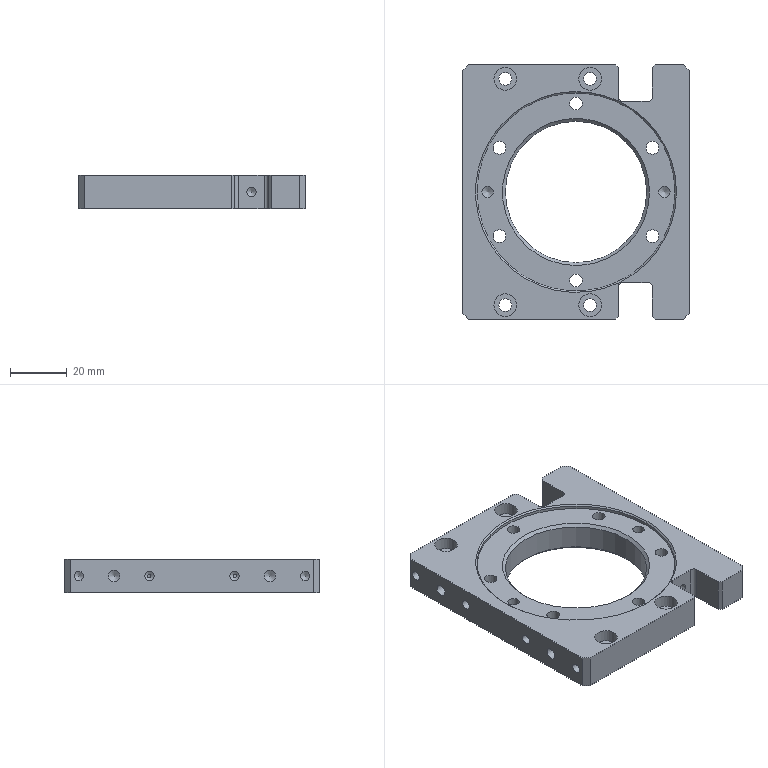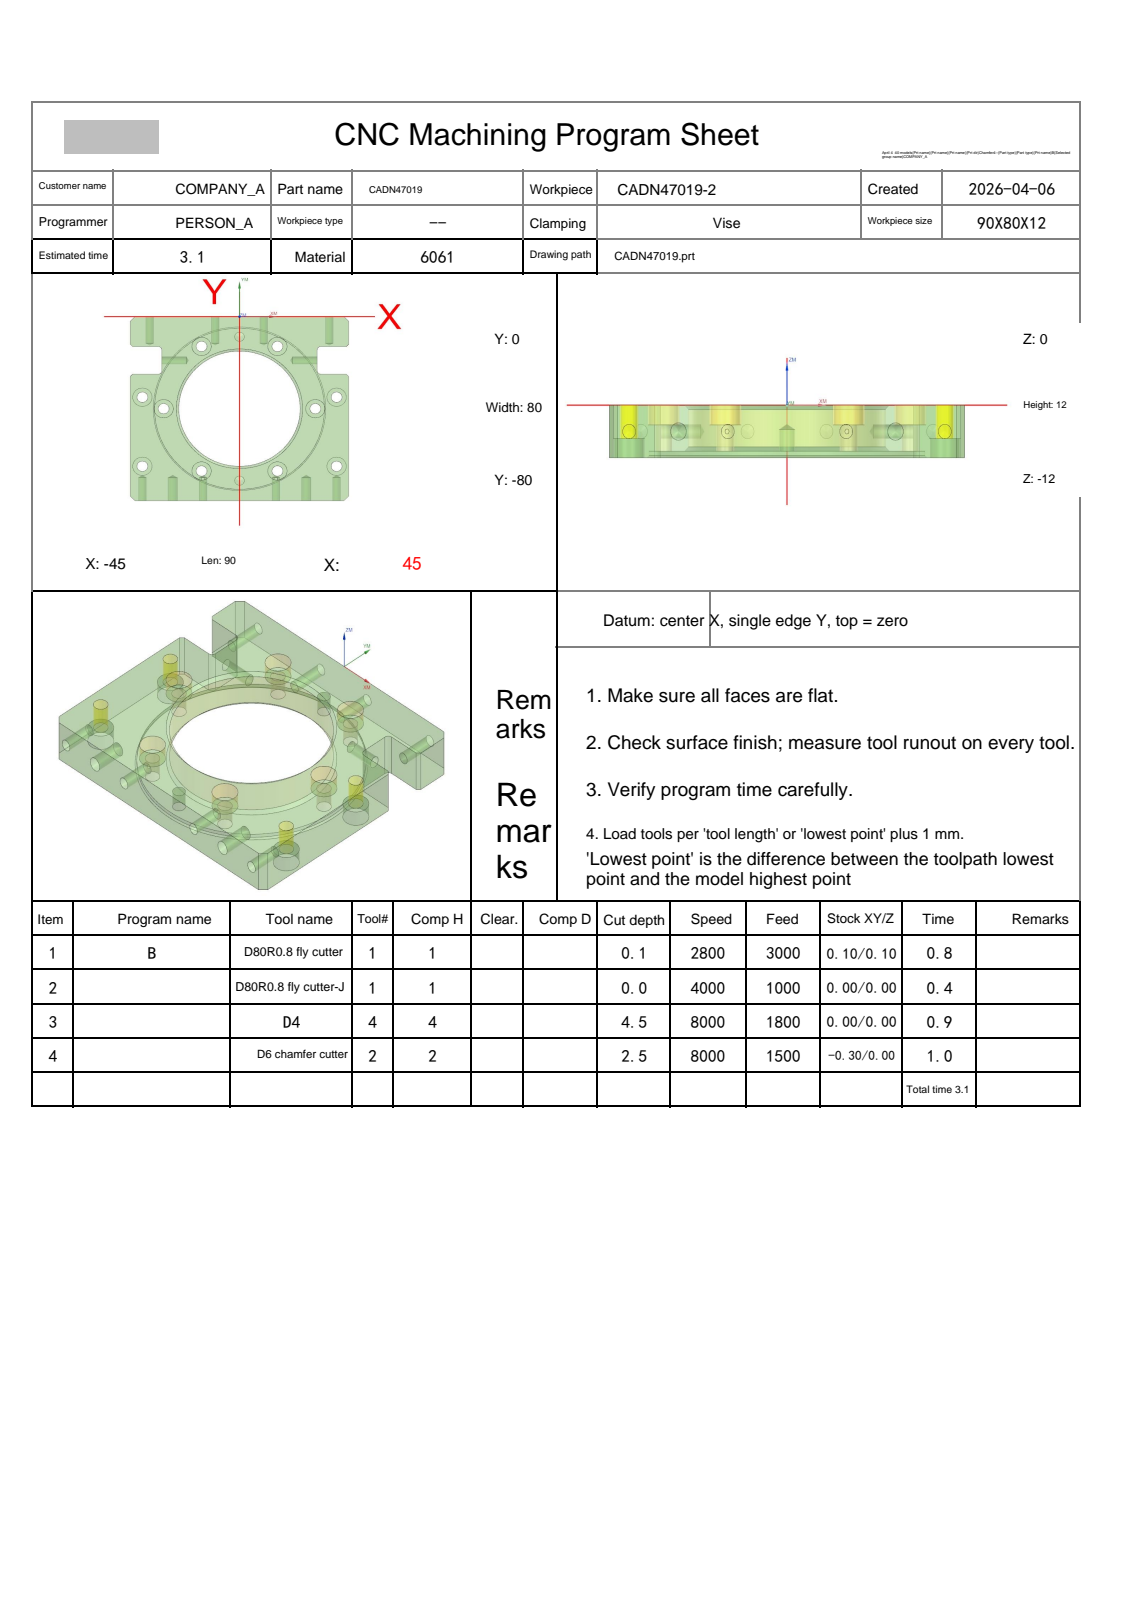NC program | NX | posted by the shop | part box 80 x 90 x 12 mm
Whole program:
%
O0001
(Machine time: 3.82 MIN)
(===Total Tool:3===)
(T1=D80R0.8 fly cutter D=80.  R=0.8  D-  H01 Z=0.    )
(T4=D4      D=4.   R=0.   D-  H04 Z=-4.5  )
(T2=D6 chamfer cutter   D=6.   R=0.   D-  H02 Z=-2.55 )
G80 G90 G17 G49 G40
G91 G28 Z0
M01
N1 T01 M06
(D80R0.8 fly cutter  D=80. R=0.8 H=01 ce=0.10 di=0.10)
G00 G90 G54 X-97.097 Y-23.903 M03 S2800
G43 H01 Z20.
M08
Z4.35
G01 Z2.35 F3000.
X-85.097
X77.897
G02 X85.097 Y-31.103 I0.0 J-7.2
G01 Y-40.737
G02 X77.097 Y-48.737 I-8. J0.0
G01 X-85.097
X-97.097
Z4.35
G00 Y-23.903
Z3.9
G01 Z1.9
X-85.097
X77.897
G02 X85.097 Y-31.103 I0.0 J-7.2
G01 Y-40.737
G02 X77.097 Y-48.737 I-8. J0.0
G01 X-85.097
X-97.097
Z3.9
G00 Y-23.903
Z3.45
G01 Z1.45
X-85.097
X77.897
G02 X85.097 Y-31.103 I0.0 J-7.2
G01 Y-40.737
G02 X77.097 Y-48.737 I-8. J0.0
G01 X-85.097
X-97.097
Z3.45
G00 Y-23.903
Z3.
G01 Z1.
X-85.097
X77.897
G02 X85.097 Y-31.103 I0.0 J-7.2
G01 Y-40.737
G02 X77.097 Y-48.737 I-8. J0.0
G01 X-85.097
X-97.097
Z3.
G00 Y-23.903
Z2.55
G01 Z.55
X-85.097
X77.897
G02 X85.097 Y-31.103 I0.0 J-7.2
G01 Y-40.737
G02 X77.097 Y-48.737 I-8. J0.0
G01 X-85.097
X-97.097
Z2.55
G00 Y-23.903
Z2.1
G01 Z.1
X-85.097
X77.897
G02 X85.097 Y-31.103 I0.0 J-7.2
G01 Y-40.737
G02 X77.097 Y-48.737 I-8. J0.0
G01 X-85.097
X-97.097
Z2.1
G00 Z20.
G91 G28 Z0.0
M05
M09
G91 G28 Z0.0
M01
N2 T01 M06
(D80R0.8 fly cutter-J  D=80. R=0.8 H=01 ce=0.00 di=0.00)
G00 G90 G54 X-96.999 Y-24.001 M03 S4000
G43 H01 Z20.
M08
Z2.
G01 Z0.0 F1000.
X-84.999
X77.002
G02 X84.999 Y-31.998 I-.003 J-8.
G01 Y-41.439
G02 X77.799 Y-48.639 I-7.2 J0.0
G01 X-84.999
X-96.999
Z2.
G00 Z20.
G91 G28 Z0.0
M05
M09
G91 G28 Z0.0
M01
N3 T04 M06
(D4  D=4. R=0. H=04 ce=0.07 di=0.00)
G00 G90 G54 X15.625 Y-12.937 M03 S8000
G43 H04 Z20.
M08
Z.3
G03 X16.59 Y-11.972 I0.0 J.965 F1800.
X15.625 Y-11.007 I-.965 J0.0
X15.625 Y-11.007 Z-.05 I0.0 J-1.93
X15.625 Y-11.007 Z-.4 I0.0 J-1.93
X15.625 Y-11.007 Z-.75 I0.0 J-1.93
X15.625 Y-11.007 Z-1.1 I0.0 J-1.93
X15.625 Y-11.007 Z-1.45 I0.0 J-1.93
X15.625 Y-11.007 Z-1.8 I0.0 J-1.93
X15.625 Y-11.007 Z-2.15 I0.0 J-1.93
X15.625 Y-11.007 Z-2.5 I0.0 J-1.93
X15.625 Y-11.007 Z-2.85 I0.0 J-1.93
X15.625 Y-11.007 Z-3.2 I0.0 J-1.93
X15.625 Y-11.007 Z-3.55 I0.0 J-1.93
X15.625 Y-11.007 Z-3.9 I0.0 J-1.93
X15.625 Y-11.007 Z-4.25 I0.0 J-1.93
X17.507 Y-13.366 Z-4.5 I0.0 J-1.93
X17.555 Y-12.937 I-1.882 J.429
X15.625 Y-11.007 I-1.93 J0.0
X13.695 Y-12.937 I0.0 J-1.93
X15.625 Y-14.867 I1.93 J0.0
X17.507 Y-13.366 I0.0 J1.93
X17.531 Y-13.151 I-.941 J.215
X16.566 Y-12.186 I-.965 J0.0
X15.625 Y-12.937 I0.0 J-.965
G00 Z20.
X-15.625
Z.3
G03 X-14.66 Y-11.972 I0.0 J.965
X-15.625 Y-11.007 I-.965 J0.0
X-15.625 Y-11.007 Z-.05 I0.0 J-1.93
X-15.625 Y-11.007 Z-.4 I0.0 J-1.93
X-15.625 Y-11.007 Z-.75 I0.0 J-1.93
X-15.625 Y-11.007 Z-1.1 I0.0 J-1.93
X-15.625 Y-11.007 Z-1.45 I0.0 J-1.93
X-15.625 Y-11.007 Z-1.8 I0.0 J-1.93
X-15.625 Y-11.007 Z-2.15 I0.0 J-1.93
X-15.625 Y-11.007 Z-2.5 I0.0 J-1.93
X-15.625 Y-11.007 Z-2.85 I0.0 J-1.93
X-15.625 Y-11.007 Z-3.2 I0.0 J-1.93
X-15.625 Y-11.007 Z-3.55 I0.0 J-1.93
X-15.625 Y-11.007 Z-3.9 I0.0 J-1.93
X-15.625 Y-11.007 Z-4.25 I0.0 J-1.93
X-13.743 Y-13.366 Z-4.5 I0.0 J-1.93
X-13.695 Y-12.937 I-1.882 J.429
X-15.625 Y-11.007 I-1.93 J0.0
X-17.555 Y-12.937 I0.0 J-1.93
X-15.625 Y-14.867 I1.93 J0.0
X-13.743 Y-13.366 I0.0 J1.93
X-13.719 Y-13.151 I-.941 J.215
X-14.684 Y-12.186 I-.965 J0.0
X-15.625 Y-12.937 I0.0 J-.965
G00 Z20.
X-31.25 Y-40.
Z.3
G03 X-30.285 Y-39.035 I0.0 J.965
X-31.25 Y-38.07 I-.965 J0.0
X-31.25 Y-38.07 Z-.05 I0.0 J-1.93
X-31.25 Y-38.07 Z-.4 I0.0 J-1.93
X-31.25 Y-38.07 Z-.75 I0.0 J-1.93
X-31.25 Y-38.07 Z-1.1 I0.0 J-1.93
X-31.25 Y-38.07 Z-1.45 I0.0 J-1.93
X-31.25 Y-38.07 Z-1.8 I0.0 J-1.93
X-31.25 Y-38.07 Z-2.15 I0.0 J-1.93
X-31.25 Y-38.07 Z-2.5 I0.0 J-1.93
X-31.25 Y-38.07 Z-2.85 I0.0 J-1.93
X-31.25 Y-38.07 Z-3.2 I0.0 J-1.93
X-31.25 Y-38.07 Z-3.55 I0.0 J-1.93
X-31.25 Y-38.07 Z-3.9 I0.0 J-1.93
X-31.25 Y-38.07 Z-4.25 I0.0 J-1.93
X-29.368 Y-40.429 Z-4.5 I0.0 J-1.93
X-29.32 Y-40. I-1.882 J.429
X-31.25 Y-38.07 I-1.93 J0.0
X-33.18 Y-40. I0.0 J-1.93
X-31.25 Y-41.93 I1.93 J0.0
X-29.368 Y-40.429 I0.0 J1.93
X-29.344 Y-40.215 I-.941 J.215
X-30.309 Y-39.25 I-.965 J0.0
X-31.25 Y-40. I0.0 J-.965
G00 Z20.
X-15.625 Y-67.063
Z.3
G03 X-14.66 Y-66.098 I0.0 J.965
X-15.625 Y-65.133 I-.965 J0.0
X-15.625 Y-65.133 Z-.05 I0.0 J-1.93
X-15.625 Y-65.133 Z-.4 I0.0 J-1.93
X-15.625 Y-65.133 Z-.75 I0.0 J-1.93
X-15.625 Y-65.133 Z-1.1 I0.0 J-1.93
X-15.625 Y-65.133 Z-1.45 I0.0 J-1.93
X-15.625 Y-65.133 Z-1.8 I0.0 J-1.93
X-15.625 Y-65.133 Z-2.15 I0.0 J-1.93
X-15.625 Y-65.133 Z-2.5 I0.0 J-1.93
X-15.625 Y-65.133 Z-2.85 I0.0 J-1.93
X-15.625 Y-65.133 Z-3.2 I0.0 J-1.93
X-15.625 Y-65.133 Z-3.55 I0.0 J-1.93
X-15.625 Y-65.133 Z-3.9 I0.0 J-1.93
X-15.625 Y-65.133 Z-4.25 I0.0 J-1.93
X-13.743 Y-67.493 Z-4.5 I0.0 J-1.93
X-13.695 Y-67.063 I-1.882 J.429
X-15.625 Y-65.133 I-1.93 J0.0
X-17.555 Y-67.063 I0.0 J-1.93
X-15.625 Y-68.993 I1.93 J0.0
X-13.743 Y-67.493 I0.0 J1.93
X-13.719 Y-67.278 I-.941 J.215
X-14.684 Y-66.313 I-.965 J0.0
X-15.625 Y-67.063 I0.0 J-.965
G00 Z20.
X15.625
Z.3
G03 X16.59 Y-66.098 I0.0 J.965
X15.625 Y-65.133 I-.965 J0.0
X15.625 Y-65.133 Z-.05 I0.0 J-1.93
X15.625 Y-65.133 Z-.4 I0.0 J-1.93
X15.625 Y-65.133 Z-.75 I0.0 J-1.93
X15.625 Y-65.133 Z-1.1 I0.0 J-1.93
X15.625 Y-65.133 Z-1.45 I0.0 J-1.93
X15.625 Y-65.133 Z-1.8 I0.0 J-1.93
X15.625 Y-65.133 Z-2.15 I0.0 J-1.93
X15.625 Y-65.133 Z-2.5 I0.0 J-1.93
X15.625 Y-65.133 Z-2.85 I0.0 J-1.93
X15.625 Y-65.133 Z-3.2 I0.0 J-1.93
X15.625 Y-65.133 Z-3.55 I0.0 J-1.93
X15.625 Y-65.133 Z-3.9 I0.0 J-1.93
X15.625 Y-65.133 Z-4.25 I0.0 J-1.93
X17.507 Y-67.493 Z-4.5 I0.0 J-1.93
X17.555 Y-67.063 I-1.882 J.429
X15.625 Y-65.133 I-1.93 J0.0
X13.695 Y-67.063 I0.0 J-1.93
X15.625 Y-68.993 I1.93 J0.0
X17.507 Y-67.493 I0.0 J1.93
X17.531 Y-67.278 I-.941 J.215
X16.566 Y-66.313 I-.965 J0.0
X15.625 Y-67.063 I0.0 J-.965
G00 Z20.
X31.25 Y-40.
Z.3
G03 X32.215 Y-39.035 I0.0 J.965
X31.25 Y-38.07 I-.965 J0.0
X31.25 Y-38.07 Z-.05 I0.0 J-1.93
X31.25 Y-38.07 Z-.4 I0.0 J-1.93
X31.25 Y-38.07 Z-.75 I0.0 J-1.93
X31.25 Y-38.07 Z-1.1 I0.0 J-1.93
X31.25 Y-38.07 Z-1.45 I0.0 J-1.93
X31.25 Y-38.07 Z-1.8 I0.0 J-1.93
X31.25 Y-38.07 Z-2.15 I0.0 J-1.93
X31.25 Y-38.07 Z-2.5 I0.0 J-1.93
X31.25 Y-38.07 Z-2.85 I0.0 J-1.93
X31.25 Y-38.07 Z-3.2 I0.0 J-1.93
X31.25 Y-38.07 Z-3.55 I0.0 J-1.93
X31.25 Y-38.07 Z-3.9 I0.0 J-1.93
X31.25 Y-38.07 Z-4.25 I0.0 J-1.93
X33.132 Y-40.429 Z-4.5 I0.0 J-1.93
X33.18 Y-40. I-1.882 J.429
X31.25 Y-38.07 I-1.93 J0.0
X29.32 Y-40. I0.0 J-1.93
X31.25 Y-41.93 I1.93 J0.0
X33.132 Y-40.429 I0.0 J1.93
X33.156 Y-40.215 I-.941 J.215
X32.191 Y-39.25 I-.965 J0.0
X31.25 Y-40. I0.0 J-.965
G00 Z20.
G00 G90 X15.625 Y-12.937 M03 S8000
Z20.
Z-4.5
G01 X15.954 Y-11.34 F600.
X15.961 Y-11.272
G03 X15.625 Y-10.937 I-.336 J0.0
X13.625 Y-12.937 I0.0 J-2.
X15.625 Y-14.937 I2. J0.0
X17.625 Y-12.937 I0.0 J2.
X15.625 Y-10.937 I-2. J0.0
X15.13 Y-10.999 I0.0 J-2.
X14.877 Y-11.324 I.083 J-.325
G01 X14.911 Y-11.471
X15.625 Y-12.937
G00 Z20.
X-15.625
Z-4.5
G01 X-15.296 Y-11.34
X-15.289 Y-11.272
G03 X-15.625 Y-10.937 I-.336 J0.0
X-17.625 Y-12.937 I0.0 J-2.
X-15.625 Y-14.937 I2. J0.0
X-13.625 Y-12.937 I0.0 J2.
X-15.625 Y-10.937 I-2. J0.0
X-16.12 Y-10.999 I0.0 J-2.
X-16.373 Y-11.324 I.083 J-.325
G01 X-16.339 Y-11.471
X-15.625 Y-12.937
G00 Z20.
X-31.25 Y-40.
Z-4.5
G01 X-30.921 Y-38.404
X-30.914 Y-38.336
G03 X-31.25 Y-38. I-.336 J0.0
X-33.25 Y-40. I0.0 J-2.
X-31.25 Y-42. I2. J0.0
X-29.25 Y-40. I0.0 J2.
X-31.25 Y-38. I-2. J0.0
X-31.745 Y-38.062 I0.0 J-2.
X-31.998 Y-38.388 I.083 J-.325
G01 X-31.964 Y-38.535
X-31.25 Y-40.
G00 Z20.
X-15.625 Y-67.063
Z-4.5
G01 X-15.296 Y-65.467
X-15.289 Y-65.399
G03 X-15.625 Y-65.063 I-.336 J0.0
X-17.625 Y-67.063 I0.0 J-2.
X-15.625 Y-69.063 I2. J0.0
X-13.625 Y-67.063 I0.0 J2.
X-15.625 Y-65.063 I-2. J0.0
X-16.12 Y-65.125 I0.0 J-2.
X-16.373 Y-65.451 I.083 J-.325
G01 X-16.339 Y-65.598
X-15.625 Y-67.063
G00 Z20.
X15.625
Z-4.5
G01 X15.954 Y-65.467
X15.961 Y-65.399
G03 X15.625 Y-65.063 I-.336 J0.0
X13.625 Y-67.063 I0.0 J-2.
X15.625 Y-69.063 I2. J0.0
X17.625 Y-67.063 I0.0 J2.
X15.625 Y-65.063 I-2. J0.0
X15.13 Y-65.125 I0.0 J-2.
X14.877 Y-65.451 I.083 J-.325
G01 X14.911 Y-65.598
X15.625 Y-67.063
G00 Z20.
X31.25 Y-40.
Z-4.5
G01 X31.579 Y-38.404
X31.586 Y-38.336
G03 X31.25 Y-38. I-.336 J0.0
X29.25 Y-40. I0.0 J-2.
X31.25 Y-42. I2. J0.0
X33.25 Y-40. I0.0 J2.
X31.25 Y-38. I-2. J0.0
X30.755 Y-38.062 I0.0 J-2.
X30.502 Y-38.388 I.083 J-.325
G01 X30.536 Y-38.535
X31.25 Y-40.
G00 Z20.
G91 G28 Z0.0
M05
M09
G91 G28 Z0.0
M01
N4 T02 M06
(D6 chamfer cutter  D=6. R=0. H=02 ce=0.00 di=0.00)
G00 G90 G54 X-40. Y-65. M03 S8000
G43 H02 Z20.
M08
G98 G81 X-40. Y-65. Z-2.55 R3. F1000.
Y-35.
X40.
Y-65.
G80
G00 Z20.
G00 G90 X-30.103 Y-39.388 M03 S8000
Z20.
Z-1.5
G01 Z-2. F600.
X-29.75 Y-39.2
G03 X-31.25 Y-37.7 I-1.5 J0.0
X-33.55 Y-40. I0.0 J-2.3
X-31.25 Y-42.3 I2.3 J0.0
X-28.95 Y-40. I0.0 J2.3
X-31.25 Y-37.7 I-2.3 J0.0
X-32.75 Y-39.2 I0.0 J-1.5
G01 X-32.397 Y-39.388
Z-1.5
G00 Z20.
X-14.478 Y-12.325
Z-1.5
G01 Z-2.
X-14.125 Y-12.137
G03 X-15.625 Y-10.637 I-1.5 J0.0
X-17.925 Y-12.937 I0.0 J-2.3
X-15.625 Y-15.237 I2.3 J0.0
X-13.325 Y-12.937 I0.0 J2.3
X-15.625 Y-10.637 I-2.3 J0.0
X-17.125 Y-12.137 I0.0 J-1.5
G01 X-16.772 Y-12.325
Z-1.5
G00 Z20.
X16.772
Z-1.5
G01 Z-2.
X17.125 Y-12.137
G03 X15.625 Y-10.637 I-1.5 J0.0
X13.325 Y-12.937 I0.0 J-2.3
X15.625 Y-15.237 I2.3 J0.0
X17.925 Y-12.937 I0.0 J2.3
X15.625 Y-10.637 I-2.3 J0.0
X14.125 Y-12.137 I0.0 J-1.5
G01 X14.478 Y-12.325
Z-1.5
G00 Z20.
X32.397 Y-39.388
Z-1.5
G01 Z-2.
X32.75 Y-39.2
G03 X31.25 Y-37.7 I-1.5 J0.0
X28.95 Y-40. I0.0 J-2.3
X31.25 Y-42.3 I2.3 J0.0
X33.55 Y-40. I0.0 J2.3
X31.25 Y-37.7 I-2.3 J0.0
X29.75 Y-39.2 I0.0 J-1.5
G01 X30.103 Y-39.388
Z-1.5
G00 Z20.
X16.772 Y-66.452
Z-1.5
G01 Z-2.
X17.125 Y-66.263
G03 X15.625 Y-64.763 I-1.5 J0.0
X13.325 Y-67.063 I0.0 J-2.3
X15.625 Y-69.363 I2.3 J0.0
X17.925 Y-67.063 I0.0 J2.3
X15.625 Y-64.763 I-2.3 J0.0
X14.125 Y-66.263 I0.0 J-1.5
G01 X14.478 Y-66.452
Z-1.5
G00 Z20.
X-14.478
Z-1.5
G01 Z-2.
X-14.125 Y-66.263
G03 X-15.625 Y-64.763 I-1.5 J0.0
X-17.925 Y-67.063 I0.0 J-2.3
X-15.625 Y-69.363 I2.3 J0.0
X-13.325 Y-67.063 I0.0 J2.3
X-15.625 Y-64.763 I-2.3 J0.0
X-17.125 Y-66.263 I0.0 J-1.5
G01 X-16.772 Y-66.452
Z-1.5
G00 Z20.
G00 G90 X1.2 Y-17.532 M03 S6500
Z20.
Z-.2
G01 Z-1.7 F1500.
Y-17.5
G03 X0.0 Y-16.3 I-1.2 J0.0
X-23.7 Y-40. I0.0 J-23.7
X0.0 Y-63.7 I23.7 J0.0
X23.158 Y-45.038 I0.0 J23.7
X23.478 Y-43.235 I-23.158 J5.038
X23.612 Y-42.036 I-23.478 J3.235
X23.638 Y-41.714 I-23.612 J2.036
X23.66 Y-41.37 I-23.638 J1.714
X23.693 Y-40.594 I-23.66 J1.37
G01 X23.696 Y-40.459
G03 X23.7 Y-40.072 I-23.695 J.459
G01 Y-40.
G03 X0.0 Y-16.3 I-23.7 J0.0
X-.4 Y-16.303 I0.0 J-23.7
X-1.58 Y-17.503 I.02 J-1.2
G01 Y-17.523
X1.2 Y-17.3
G03 X0.0 Y-16.1 I-1.2 J0.0
X-23.9 Y-40. I0.0 J-23.9
X0.0 Y-63.9 I23.9 J0.0
X23.354 Y-45.08 I0.0 J23.9
X23.676 Y-43.262 I-23.354 J5.08
X23.812 Y-42.053 I-23.676 J3.262
X23.837 Y-41.729 I-23.812 J2.053
X23.86 Y-41.381 I-23.837 J1.729
X23.892 Y-40.599 I-23.86 J1.381
G01 X23.896 Y-40.463
G03 X23.9 Y-40.072 I-23.895 J.463
G01 Y-40.
G03 X0.0 Y-16.1 I-23.9 J0.0
X-.4 Y-16.103 I0.0 J-23.9
X-1.58 Y-17.303 I.02 J-1.2
G01 Y-17.323
X1.2 Y-17.1
G03 X0.0 Y-15.9 I-1.2 J0.0
X-24.1 Y-40. I0.0 J-24.1
X0.0 Y-64.1 I24.1 J0.0
X23.549 Y-45.123 I0.0 J24.1
X23.874 Y-43.29 I-23.549 J5.123
X24.011 Y-42.07 I-23.874 J3.29
X24.037 Y-41.743 I-24.011 J2.07
X24.06 Y-41.393 I-24.037 J1.743
X24.092 Y-40.604 I-24.06 J1.393
G01 X24.095 Y-40.467
G03 X24.1 Y-40.073 I-24.095 J.467
G01 Y-40.
G03 X0.0 Y-15.9 I-24.1 J0.0
X-.4 Y-15.903 I0.0 J-24.1
X-1.58 Y-17.103 I.02 J-1.2
G01 Y-17.123
X1.2 Y-16.9
G03 X0.0 Y-15.7 I-1.2 J0.0
X-24.3 Y-40. I0.0 J-24.3
X0.0 Y-64.3 I24.3 J0.0
X23.745 Y-45.165 I0.0 J24.3
X24.073 Y-43.317 I-23.745 J5.165
X24.21 Y-42.088 I-24.073 J3.317
X24.236 Y-41.758 I-24.21 J2.088
X24.259 Y-41.404 I-24.236 J1.758
X24.292 Y-40.609 I-24.259 J1.404
G01 X24.295 Y-40.471
G03 X24.3 Y-40.073 I-24.295 J.471
G01 Y-40.
G03 X0.0 Y-15.7 I-24.3 J0.0
X-.4 Y-15.703 I0.0 J-24.3
X-1.58 Y-16.903 I.02 J-1.2
G01 Y-16.923
Y-16.954
Z-.2
G00 Z20.
G00 G90 X-36.998 Y-13.7 M03 S7000
Z20.
Z2.5
G01 X-43.953 Z-.031 F1500.
X-44.16 Y-13.662 Z-.108
X-44.355 Y-13.581 Z-.185
X-44.528 Y-13.462 Z-.261
X-45.462 Y-12.528 Z-.742
X-45.581 Y-12.355 Z-.819
X-45.662 Y-12.16 Z-.895
X-45.7 Y-11.953 Z-.972
Y-11.876 Z-1.
Y-2.124
G02 X-45.407 Y-1.417 I1. J0.0
G01 X-43.583 Y.407
G02 X-42.876 Y.7 I.707 J-.707
G01 X42.876
G02 X43.583 Y.407 I0.0 J-1.
G01 X45.407 Y-1.417
G02 X45.7 Y-2.124 I-.707 J-.707
G01 Y-11.876
G02 X45.407 Y-12.583 I-1. J0.0
G01 X44.583 Y-13.407
G02 X43.876 Y-13.7 I-.707 J.707
G01 X33.5
G03 X32.7 Y-14.5 I0.0 J-.8
G01 Y-23.5
G03 X33.5 Y-24.3 I.8 J0.0
G01 X43.876
G02 X44.583 Y-24.593 I0.0 J-1.
G01 X45.407 Y-25.417
G02 X45.7 Y-26.124 I-.707 J-.707
G01 Y-77.876
G02 X45.407 Y-78.583 I-1. J0.0
G01 X43.583 Y-80.407
G02 X42.876 Y-80.7 I-.707 J.707
G01 X-42.876
G02 X-43.583 Y-80.407 I0.0 J1.
G01 X-45.407 Y-78.583
G02 X-45.7 Y-77.876 I.707 J.707
G01 Y-26.124
G02 X-45.407 Y-25.417 I1. J0.0
G01 X-44.583 Y-24.593
G02 X-43.876 Y-24.3 I.707 J-.707
G01 X-33.5
G03 X-32.7 Y-23.5 I0.0 J.8
G01 Y-14.5
G03 X-33.5 Y-13.7 I-.8 J0.0
G01 X-43.876
G02 X-44.583 Y-13.407 I0.0 J1.
G01 X-45.407 Y-12.583
G02 X-45.7 Y-11.876 I.707 J.707
G01 Y-11.376
Z1.5
G00 Z20.
M05
M09
G91 G28 Z0.0
G91 G28 Y0.0
M30
%